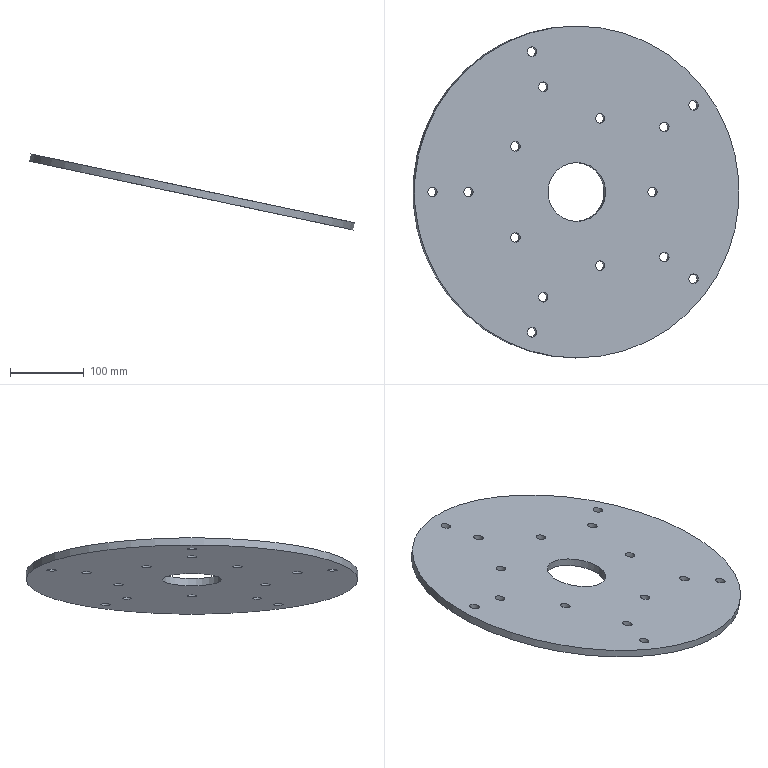Part | STEP file | HL4GZ-1.862.631 (blade mounting disc) | 1 solid | 19 faces | box 442.246 x 450 x 103.342 mm | volume 1520256 mm3 | cylinder 17 | plane 2 | commonest cylinder face diameters 13 x15 80 x1 450 x1